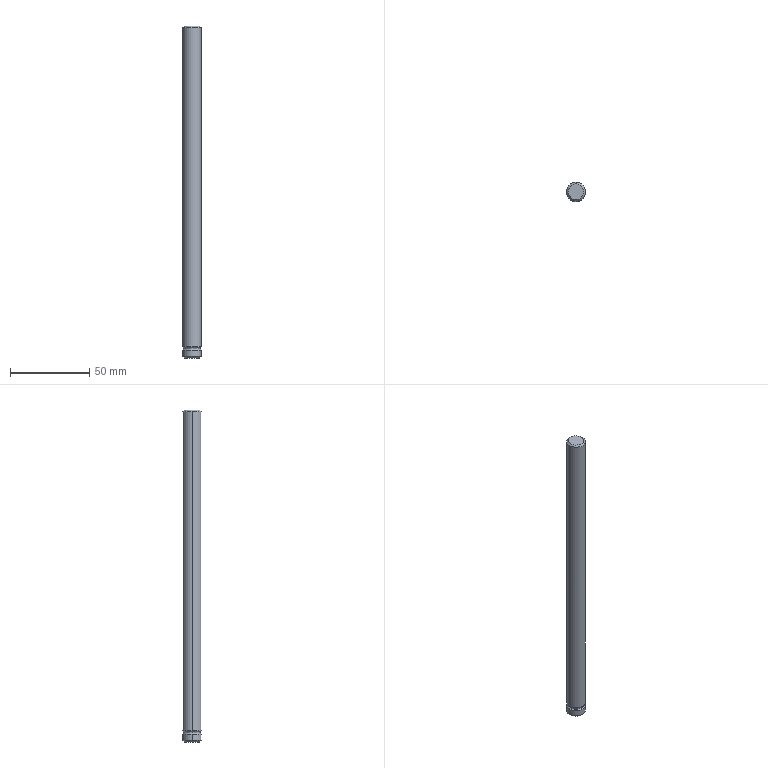Part | STEP file | Rotor mis-part check fixture-guide rod | 1 solid | 16 faces | box 12 x 12 x 210 mm | volume 23681 mm3 | cone 8 | cylinder 4 | spline 2 | plane 2 | commonest cylinder face diameters 12 x4
STEP:
#1=CARTESIAN_POINT('',(0.,0.,0.));
#2=DIRECTION('',(0.,0.,1.));
#3=DIRECTION('',(1.,0.,0.));
#4=AXIS2_PLACEMENT_3D('',#1,#2,#3);
#5=CARTESIAN_POINT('',(-5.354,0.,6.354));
#6=VERTEX_POINT('',#5);
#7=CARTESIAN_POINT('',(-5.354,0.,5.646));
#8=VERTEX_POINT('',#7);
#9=CARTESIAN_POINT('',(-5.707,0.,6.));
#10=DIRECTION('',(0.,1.,0.));
#11=DIRECTION('',(-1.,0.,0.));
#12=AXIS2_PLACEMENT_3D('',#9,#10,#11);
#13=CIRCLE('',#12,0.5);
#14=CARTESIAN_POINT('',(-5.354,0.,6.354));
#15=CARTESIAN_POINT('',(-5.354,10.707,6.354));
#16=CARTESIAN_POINT('',(5.354,10.707,6.354));
#17=CARTESIAN_POINT('',(5.354,0.,6.354));
#18=CARTESIAN_POINT('',(-5.146,0.,6.146));
#19=CARTESIAN_POINT('',(-5.146,10.293,6.146));
#20=CARTESIAN_POINT('',(5.146,10.293,6.146));
#21=CARTESIAN_POINT('',(5.146,0.,6.146));
#22=CARTESIAN_POINT('',(-5.146,0.,5.854));
#23=CARTESIAN_POINT('',(-5.146,10.293,5.854));
#24=CARTESIAN_POINT('',(5.146,10.293,5.854));
#25=CARTESIAN_POINT('',(5.146,0.,5.854));
#26=CARTESIAN_POINT('',(-5.354,0.,5.646));
#27=CARTESIAN_POINT('',(-5.354,10.707,5.646));
#28=CARTESIAN_POINT('',(5.354,10.707,5.646));
#29=CARTESIAN_POINT('',(5.354,0.,5.646));
#30=(BOUNDED_SURFACE()B_SPLINE_SURFACE(3,3,((#14,#15,#16,#17),(#18,#19,#20,#21),(#22,#23,#24,#25),(#26,#27,#28,#29)),.UNSPECIFIED.,.F.,.F.,.F.)B_SPLINE_SURFACE_WITH_KNOTS((4,4),(4,4),(0.,1.),(0.,1.),.PIECEWISE_BEZIER_KNOTS.)GEOMETRIC_REPRESENTATION_ITEM()RATIONAL_B_SPLINE_SURFACE(((1.,0.3333,0.3333,1.),(0.8047,0.2682,0.2682,0.8047),(0.8047,0.2682,0.2682,0.8047),(1.,0.3333,0.3333,1.)))REPRESENTATION_ITEM('')SURFACE());
#31=CARTESIAN_POINT('',(0.,0.));
#32=CARTESIAN_POINT('',(0.01683,0.));
#33=CARTESIAN_POINT('',(0.04999,0.));
#34=CARTESIAN_POINT('',(0.09843,0.));
#35=CARTESIAN_POINT('',(0.1457,0.));
#36=CARTESIAN_POINT('',(0.192,0.));
#37=CARTESIAN_POINT('',(0.2375,0.));
#38=CARTESIAN_POINT('',(0.2823,0.));
#39=CARTESIAN_POINT('',(0.3265,0.));
#40=CARTESIAN_POINT('',(0.3703,0.));
#41=CARTESIAN_POINT('',(0.4137,0.));
#42=CARTESIAN_POINT('',(0.4569,0.));
#43=CARTESIAN_POINT('',(0.5,0.));
#44=CARTESIAN_POINT('',(0.5431,0.));
#45=CARTESIAN_POINT('',(0.5863,0.));
#46=CARTESIAN_POINT('',(0.6297,0.));
#47=CARTESIAN_POINT('',(0.6735,0.));
#48=CARTESIAN_POINT('',(0.7177,0.));
#49=CARTESIAN_POINT('',(0.7625,0.));
#50=CARTESIAN_POINT('',(0.808,0.));
#51=CARTESIAN_POINT('',(0.8543,0.));
#52=CARTESIAN_POINT('',(0.9016,0.));
#53=CARTESIAN_POINT('',(0.95,0.));
#54=CARTESIAN_POINT('',(0.9832,0.));
#55=CARTESIAN_POINT('',(1.,0.));
#56=B_SPLINE_CURVE_WITH_KNOTS('',3,(#31,#32,#33,#34,#35,#36,#37,#38,#39,#40,#41,#42,#43,#44,#45,#46,#47,#48,#49,#50,#51,#52,#53,#54,#55),.UNSPECIFIED.,.F.,.F.,(4,1,1,1,1,1,1,1,1,1,1,1,1,1,1,1,1,1,1,1,1,1,4),(2.356,2.428,2.499,2.57,2.642,2.713,2.785,2.856,2.927,2.999,3.07,3.142,3.213,3.284,3.356,3.427,3.499,3.57,3.641,3.713,3.784,3.856,3.927),.QUASI_UNIFORM_KNOTS.);
#57=(GEOMETRIC_REPRESENTATION_CONTEXT(2)PARAMETRIC_REPRESENTATION_CONTEXT()REPRESENTATION_CONTEXT('',''));
#58=DEFINITIONAL_REPRESENTATION('',(#56),#57);
#59=PCURVE('',#30,#58);
#60=CARTESIAN_POINT('',(5.354,0.,6.354));
#61=CARTESIAN_POINT('',(5.354,-10.707,6.354));
#62=CARTESIAN_POINT('',(-5.354,-10.707,6.354));
#63=CARTESIAN_POINT('',(-5.354,0.,6.354));
#64=CARTESIAN_POINT('',(5.146,0.,6.146));
#65=CARTESIAN_POINT('',(5.146,-10.293,6.146));
#66=CARTESIAN_POINT('',(-5.146,-10.293,6.146));
#67=CARTESIAN_POINT('',(-5.146,0.,6.146));
#68=CARTESIAN_POINT('',(5.146,0.,5.854));
#69=CARTESIAN_POINT('',(5.146,-10.293,5.854));
#70=CARTESIAN_POINT('',(-5.146,-10.293,5.854));
#71=CARTESIAN_POINT('',(-5.146,0.,5.854));
#72=CARTESIAN_POINT('',(5.354,0.,5.646));
#73=CARTESIAN_POINT('',(5.354,-10.707,5.646));
#74=CARTESIAN_POINT('',(-5.354,-10.707,5.646));
#75=CARTESIAN_POINT('',(-5.354,0.,5.646));
#76=(BOUNDED_SURFACE()B_SPLINE_SURFACE(3,3,((#60,#61,#62,#63),(#64,#65,#66,#67),(#68,#69,#70,#71),(#72,#73,#74,#75)),.UNSPECIFIED.,.F.,.F.,.F.)B_SPLINE_SURFACE_WITH_KNOTS((4,4),(4,4),(0.,1.),(0.,1.),.PIECEWISE_BEZIER_KNOTS.)GEOMETRIC_REPRESENTATION_ITEM()RATIONAL_B_SPLINE_SURFACE(((1.,0.3333,0.3333,1.),(0.8047,0.2682,0.2682,0.8047),(0.8047,0.2682,0.2682,0.8047),(1.,0.3333,0.3333,1.)))REPRESENTATION_ITEM('')SURFACE());
#77=CARTESIAN_POINT('',(0.,1.));
#78=CARTESIAN_POINT('',(0.01683,1.));
#79=CARTESIAN_POINT('',(0.04999,1.));
#80=CARTESIAN_POINT('',(0.09843,1.));
#81=CARTESIAN_POINT('',(0.1457,1.));
#82=CARTESIAN_POINT('',(0.192,1.));
#83=CARTESIAN_POINT('',(0.2375,1.));
#84=CARTESIAN_POINT('',(0.2823,1.));
#85=CARTESIAN_POINT('',(0.3265,1.));
#86=CARTESIAN_POINT('',(0.3703,1.));
#87=CARTESIAN_POINT('',(0.4137,1.));
#88=CARTESIAN_POINT('',(0.4569,1.));
#89=CARTESIAN_POINT('',(0.5,1.));
#90=CARTESIAN_POINT('',(0.5431,1.));
#91=CARTESIAN_POINT('',(0.5863,1.));
#92=CARTESIAN_POINT('',(0.6297,1.));
#93=CARTESIAN_POINT('',(0.6735,1.));
#94=CARTESIAN_POINT('',(0.7177,1.));
#95=CARTESIAN_POINT('',(0.7625,1.));
#96=CARTESIAN_POINT('',(0.808,1.));
#97=CARTESIAN_POINT('',(0.8543,1.));
#98=CARTESIAN_POINT('',(0.9016,1.));
#99=CARTESIAN_POINT('',(0.95,1.));
#100=CARTESIAN_POINT('',(0.9832,1.));
#101=CARTESIAN_POINT('',(1.,1.));
#102=B_SPLINE_CURVE_WITH_KNOTS('',3,(#77,#78,#79,#80,#81,#82,#83,#84,#85,#86,#87,#88,#89,#90,#91,#92,#93,#94,#95,#96,#97,#98,#99,#100,#101),.UNSPECIFIED.,.F.,.F.,(4,1,1,1,1,1,1,1,1,1,1,1,1,1,1,1,1,1,1,1,1,1,4),(2.356,2.428,2.499,2.57,2.642,2.713,2.785,2.856,2.927,2.999,3.07,3.142,3.213,3.284,3.356,3.427,3.499,3.57,3.641,3.713,3.784,3.856,3.927),.QUASI_UNIFORM_KNOTS.);
#103=(GEOMETRIC_REPRESENTATION_CONTEXT(2)PARAMETRIC_REPRESENTATION_CONTEXT()REPRESENTATION_CONTEXT('',''));
#104=DEFINITIONAL_REPRESENTATION('',(#102),#103);
#105=PCURVE('',#76,#104);
#106=SURFACE_CURVE('',#13,(#59,#105),.PCURVE_S1.);
#107=EDGE_CURVE('',#6,#8,#106,.T.);
#108=ORIENTED_EDGE('',*,*,#107,.T.);
#109=CARTESIAN_POINT('',(5.354,0.,5.646));
#110=VERTEX_POINT('',#109);
#111=CARTESIAN_POINT('',(0.,0.,5.646));
#112=DIRECTION('',(0.,0.,-1.));
#113=DIRECTION('',(-1.,0.,0.));
#114=AXIS2_PLACEMENT_3D('',#111,#112,#113);
#115=CIRCLE('',#114,5.354);
#116=CARTESIAN_POINT('',(1.,0.));
#117=CARTESIAN_POINT('',(1.,0.02375));
#118=CARTESIAN_POINT('',(1.,0.06805));
#119=CARTESIAN_POINT('',(1.,0.1267));
#120=CARTESIAN_POINT('',(1.,0.1794));
#121=CARTESIAN_POINT('',(1.,0.2276));
#122=CARTESIAN_POINT('',(1.,0.2721));
#123=CARTESIAN_POINT('',(1.,0.3139));
#124=CARTESIAN_POINT('',(1.,0.3535));
#125=CARTESIAN_POINT('',(1.,0.3914));
#126=CARTESIAN_POINT('',(1.,0.4282));
#127=CARTESIAN_POINT('',(1.,0.4643));
#128=CARTESIAN_POINT('',(1.,0.5));
#129=CARTESIAN_POINT('',(1.,0.5357));
#130=CARTESIAN_POINT('',(1.,0.5718));
#131=CARTESIAN_POINT('',(1.,0.6086));
#132=CARTESIAN_POINT('',(1.,0.6465));
#133=CARTESIAN_POINT('',(1.,0.6861));
#134=CARTESIAN_POINT('',(1.,0.7279));
#135=CARTESIAN_POINT('',(1.,0.7724));
#136=CARTESIAN_POINT('',(1.,0.8206));
#137=CARTESIAN_POINT('',(1.,0.8733));
#138=CARTESIAN_POINT('',(1.,0.9319));
#139=CARTESIAN_POINT('',(1.,0.9763));
#140=CARTESIAN_POINT('',(1.,1.));
#141=B_SPLINE_CURVE_WITH_KNOTS('',3,(#116,#117,#118,#119,#120,#121,#122,#123,#124,#125,#126,#127,#128,#129,#130,#131,#132,#133,#134,#135,#136,#137,#138,#139,#140),.UNSPECIFIED.,.F.,.F.,(4,1,1,1,1,1,1,1,1,1,1,1,1,1,1,1,1,1,1,1,1,1,4),(0.,0.1428,0.2856,0.4284,0.5712,0.714,0.8568,0.9996,1.142,1.285,1.428,1.571,1.714,1.856,1.999,2.142,2.285,2.428,2.57,2.713,2.856,2.999,3.142),.QUASI_UNIFORM_KNOTS.);
#142=(GEOMETRIC_REPRESENTATION_CONTEXT(2)PARAMETRIC_REPRESENTATION_CONTEXT()REPRESENTATION_CONTEXT('',''));
#143=DEFINITIONAL_REPRESENTATION('',(#141),#142);
#144=PCURVE('',#30,#143);
#145=CARTESIAN_POINT('',(0.,0.,5.));
#146=DIRECTION('',(0.,0.,-1.));
#147=DIRECTION('',(-1.,0.,0.));
#148=AXIS2_PLACEMENT_3D('',#145,#146,#147);
#149=CONICAL_SURFACE('',#148,6.,0.7854);
#150=CARTESIAN_POINT('',(0.,-0.6464));
#151=DIRECTION('',(1.,0.));
#152=VECTOR('',#151,1.);
#153=LINE('',#150,#152);
#154=(GEOMETRIC_REPRESENTATION_CONTEXT(2)PARAMETRIC_REPRESENTATION_CONTEXT()REPRESENTATION_CONTEXT('',''));
#155=DEFINITIONAL_REPRESENTATION('',(#153),#154);
#156=PCURVE('',#149,#155);
#157=SURFACE_CURVE('',#115,(#144,#156),.PCURVE_S1.);
#158=EDGE_CURVE('',#8,#110,#157,.T.);
#159=ORIENTED_EDGE('',*,*,#158,.T.);
#160=CARTESIAN_POINT('',(5.354,0.,6.354));
#161=VERTEX_POINT('',#160);
#162=CARTESIAN_POINT('',(5.707,0.,6.));
#163=DIRECTION('',(0.,-1.,0.));
#164=DIRECTION('',(1.,0.,0.));
#165=AXIS2_PLACEMENT_3D('',#162,#163,#164);
#166=CIRCLE('',#165,0.5);
#167=CARTESIAN_POINT('',(0.,1.));
#168=CARTESIAN_POINT('',(0.01683,1.));
#169=CARTESIAN_POINT('',(0.04999,1.));
#170=CARTESIAN_POINT('',(0.09843,1.));
#171=CARTESIAN_POINT('',(0.1457,1.));
#172=CARTESIAN_POINT('',(0.192,1.));
#173=CARTESIAN_POINT('',(0.2375,1.));
#174=CARTESIAN_POINT('',(0.2823,1.));
#175=CARTESIAN_POINT('',(0.3265,1.));
#176=CARTESIAN_POINT('',(0.3703,1.));
#177=CARTESIAN_POINT('',(0.4137,1.));
#178=CARTESIAN_POINT('',(0.4569,1.));
#179=CARTESIAN_POINT('',(0.5,1.));
#180=CARTESIAN_POINT('',(0.5431,1.));
#181=CARTESIAN_POINT('',(0.5863,1.));
#182=CARTESIAN_POINT('',(0.6297,1.));
#183=CARTESIAN_POINT('',(0.6735,1.));
#184=CARTESIAN_POINT('',(0.7177,1.));
#185=CARTESIAN_POINT('',(0.7625,1.));
#186=CARTESIAN_POINT('',(0.808,1.));
#187=CARTESIAN_POINT('',(0.8543,1.));
#188=CARTESIAN_POINT('',(0.9016,1.));
#189=CARTESIAN_POINT('',(0.95,1.));
#190=CARTESIAN_POINT('',(0.9832,1.));
#191=CARTESIAN_POINT('',(1.,1.));
#192=B_SPLINE_CURVE_WITH_KNOTS('',3,(#167,#168,#169,#170,#171,#172,#173,#174,#175,#176,#177,#178,#179,#180,#181,#182,#183,#184,#185,#186,#187,#188,#189,#190,#191),.UNSPECIFIED.,.F.,.F.,(4,1,1,1,1,1,1,1,1,1,1,1,1,1,1,1,1,1,1,1,1,1,4),(2.356,2.428,2.499,2.57,2.642,2.713,2.785,2.856,2.927,2.999,3.07,3.142,3.213,3.284,3.356,3.427,3.499,3.57,3.641,3.713,3.784,3.856,3.927),.QUASI_UNIFORM_KNOTS.);
#193=(GEOMETRIC_REPRESENTATION_CONTEXT(2)PARAMETRIC_REPRESENTATION_CONTEXT()REPRESENTATION_CONTEXT('',''));
#194=DEFINITIONAL_REPRESENTATION('',(#192),#193);
#195=PCURVE('',#30,#194);
#196=CARTESIAN_POINT('',(0.,0.));
#197=CARTESIAN_POINT('',(0.01683,0.));
#198=CARTESIAN_POINT('',(0.04999,0.));
#199=CARTESIAN_POINT('',(0.09843,0.));
#200=CARTESIAN_POINT('',(0.1457,0.));
#201=CARTESIAN_POINT('',(0.192,0.));
#202=CARTESIAN_POINT('',(0.2375,0.));
#203=CARTESIAN_POINT('',(0.2823,0.));
#204=CARTESIAN_POINT('',(0.3265,0.));
#205=CARTESIAN_POINT('',(0.3703,0.));
#206=CARTESIAN_POINT('',(0.4137,0.));
#207=CARTESIAN_POINT('',(0.4569,0.));
#208=CARTESIAN_POINT('',(0.5,0.));
#209=CARTESIAN_POINT('',(0.5431,0.));
#210=CARTESIAN_POINT('',(0.5863,0.));
#211=CARTESIAN_POINT('',(0.6297,0.));
#212=CARTESIAN_POINT('',(0.6735,0.));
#213=CARTESIAN_POINT('',(0.7177,0.));
#214=CARTESIAN_POINT('',(0.7625,0.));
#215=CARTESIAN_POINT('',(0.808,0.));
#216=CARTESIAN_POINT('',(0.8543,0.));
#217=CARTESIAN_POINT('',(0.9016,0.));
#218=CARTESIAN_POINT('',(0.95,0.));
#219=CARTESIAN_POINT('',(0.9832,0.));
#220=CARTESIAN_POINT('',(1.,0.));
#221=B_SPLINE_CURVE_WITH_KNOTS('',3,(#196,#197,#198,#199,#200,#201,#202,#203,#204,#205,#206,#207,#208,#209,#210,#211,#212,#213,#214,#215,#216,#217,#218,#219,#220),.UNSPECIFIED.,.F.,.F.,(4,1,1,1,1,1,1,1,1,1,1,1,1,1,1,1,1,1,1,1,1,1,4),(2.356,2.428,2.499,2.57,2.642,2.713,2.785,2.856,2.927,2.999,3.07,3.142,3.213,3.284,3.356,3.427,3.499,3.57,3.641,3.713,3.784,3.856,3.927),.QUASI_UNIFORM_KNOTS.);
#222=(GEOMETRIC_REPRESENTATION_CONTEXT(2)PARAMETRIC_REPRESENTATION_CONTEXT()REPRESENTATION_CONTEXT('',''));
#223=DEFINITIONAL_REPRESENTATION('',(#221),#222);
#224=PCURVE('',#76,#223);
#225=SURFACE_CURVE('',#166,(#195,#224),.PCURVE_S1.);
#226=EDGE_CURVE('',#161,#110,#225,.T.);
#227=ORIENTED_EDGE('',*,*,#226,.F.);
#228=CARTESIAN_POINT('',(0.,0.,6.354));
#229=DIRECTION('',(0.,0.,1.));
#230=DIRECTION('',(1.,0.,0.));
#231=AXIS2_PLACEMENT_3D('',#228,#229,#230);
#232=CIRCLE('',#231,5.354);
#233=CARTESIAN_POINT('',(0.,1.));
#234=CARTESIAN_POINT('',(0.,0.9763));
#235=CARTESIAN_POINT('',(0.,0.9319));
#236=CARTESIAN_POINT('',(0.,0.8733));
#237=CARTESIAN_POINT('',(0.,0.8206));
#238=CARTESIAN_POINT('',(0.,0.7724));
#239=CARTESIAN_POINT('',(0.,0.7279));
#240=CARTESIAN_POINT('',(0.,0.6861));
#241=CARTESIAN_POINT('',(0.,0.6465));
#242=CARTESIAN_POINT('',(0.,0.6086));
#243=CARTESIAN_POINT('',(0.,0.5718));
#244=CARTESIAN_POINT('',(0.,0.5357));
#245=CARTESIAN_POINT('',(0.,0.5));
#246=CARTESIAN_POINT('',(0.,0.4643));
#247=CARTESIAN_POINT('',(0.,0.4282));
#248=CARTESIAN_POINT('',(0.,0.3914));
#249=CARTESIAN_POINT('',(0.,0.3535));
#250=CARTESIAN_POINT('',(0.,0.3139));
#251=CARTESIAN_POINT('',(0.,0.2721));
#252=CARTESIAN_POINT('',(0.,0.2276));
#253=CARTESIAN_POINT('',(0.,0.1794));
#254=CARTESIAN_POINT('',(0.,0.1267));
#255=CARTESIAN_POINT('',(0.,0.06805));
#256=CARTESIAN_POINT('',(0.,0.02375));
#257=CARTESIAN_POINT('',(0.,0.));
#258=B_SPLINE_CURVE_WITH_KNOTS('',3,(#233,#234,#235,#236,#237,#238,#239,#240,#241,#242,#243,#244,#245,#246,#247,#248,#249,#250,#251,#252,#253,#254,#255,#256,#257),.UNSPECIFIED.,.F.,.F.,(4,1,1,1,1,1,1,1,1,1,1,1,1,1,1,1,1,1,1,1,1,1,4),(0.,0.1428,0.2856,0.4284,0.5712,0.714,0.8568,0.9996,1.142,1.285,1.428,1.571,1.714,1.856,1.999,2.142,2.285,2.428,2.57,2.713,2.856,2.999,3.142),.QUASI_UNIFORM_KNOTS.);
#259=(GEOMETRIC_REPRESENTATION_CONTEXT(2)PARAMETRIC_REPRESENTATION_CONTEXT()REPRESENTATION_CONTEXT('',''));
#260=DEFINITIONAL_REPRESENTATION('',(#258),#259);
#261=PCURVE('',#30,#260);
#262=CARTESIAN_POINT('',(0.,0.,7.));
#263=DIRECTION('',(0.,0.,1.));
#264=DIRECTION('',(1.,0.,0.));
#265=AXIS2_PLACEMENT_3D('',#262,#263,#264);
#266=CONICAL_SURFACE('',#265,6.,0.7854);
#267=CARTESIAN_POINT('',(0.,-0.6464));
#268=DIRECTION('',(1.,0.));
#269=VECTOR('',#268,1.);
#270=LINE('',#267,#269);
#271=(GEOMETRIC_REPRESENTATION_CONTEXT(2)PARAMETRIC_REPRESENTATION_CONTEXT()REPRESENTATION_CONTEXT('',''));
#272=DEFINITIONAL_REPRESENTATION('',(#270),#271);
#273=PCURVE('',#266,#272);
#274=SURFACE_CURVE('',#232,(#261,#273),.PCURVE_S1.);
#275=EDGE_CURVE('',#161,#6,#274,.T.);
#276=ORIENTED_EDGE('',*,*,#275,.T.);
#277=EDGE_LOOP('',(#108,#159,#227,#276));
#278=FACE_BOUND('',#277,.F.);
#279=ADVANCED_FACE('',(#278),#30,.F.);
#280=CARTESIAN_POINT('',(-6.,0.,209.));
#281=VERTEX_POINT('',#280);
#282=CARTESIAN_POINT('',(6.,0.,209.));
#283=VERTEX_POINT('',#282);
#284=CARTESIAN_POINT('',(0.,0.,209.));
#285=DIRECTION('',(0.,0.,-1.));
#286=DIRECTION('',(-1.,0.,0.));
#287=AXIS2_PLACEMENT_3D('',#284,#285,#286);
#288=CIRCLE('',#287,6.);
#289=CARTESIAN_POINT('',(0.,0.,210.));
#290=DIRECTION('',(0.,0.,-1.));
#291=DIRECTION('',(-1.,0.,0.));
#292=AXIS2_PLACEMENT_3D('',#289,#290,#291);
#293=CYLINDRICAL_SURFACE('',#292,6.);
#294=CARTESIAN_POINT('',(0.,1.));
#295=DIRECTION('',(1.,0.));
#296=VECTOR('',#295,1.);
#297=LINE('',#294,#296);
#298=(GEOMETRIC_REPRESENTATION_CONTEXT(2)PARAMETRIC_REPRESENTATION_CONTEXT()REPRESENTATION_CONTEXT('',''));
#299=DEFINITIONAL_REPRESENTATION('',(#297),#298);
#300=PCURVE('',#293,#299);
#301=CARTESIAN_POINT('',(0.,0.,209.));
#302=DIRECTION('',(0.,0.,-1.));
#303=DIRECTION('',(-1.,0.,0.));
#304=AXIS2_PLACEMENT_3D('',#301,#302,#303);
#305=CONICAL_SURFACE('',#304,6.,0.7854);
#306=CARTESIAN_POINT('',(0.,0.));
#307=DIRECTION('',(1.,0.));
#308=VECTOR('',#307,1.);
#309=LINE('',#306,#308);
#310=(GEOMETRIC_REPRESENTATION_CONTEXT(2)PARAMETRIC_REPRESENTATION_CONTEXT()REPRESENTATION_CONTEXT('',''));
#311=DEFINITIONAL_REPRESENTATION('',(#309),#310);
#312=PCURVE('',#305,#311);
#313=SURFACE_CURVE('',#288,(#300,#312),.PCURVE_S1.);
#314=EDGE_CURVE('',#281,#283,#313,.T.);
#315=ORIENTED_EDGE('',*,*,#314,.T.);
#316=CARTESIAN_POINT('',(6.,0.,7.));
#317=VERTEX_POINT('',#316);
#318=CARTESIAN_POINT('',(6.,0.,210.));
#319=DIRECTION('',(0.,0.,-1.));
#320=VECTOR('',#319,1.);
#321=LINE('',#318,#320);
#322=CARTESIAN_POINT('',(3.142,0.));
#323=DIRECTION('',(0.,1.));
#324=VECTOR('',#323,1.);
#325=LINE('',#322,#324);
#326=(GEOMETRIC_REPRESENTATION_CONTEXT(2)PARAMETRIC_REPRESENTATION_CONTEXT()REPRESENTATION_CONTEXT('',''));
#327=DEFINITIONAL_REPRESENTATION('',(#325),#326);
#328=PCURVE('',#293,#327);
#329=CARTESIAN_POINT('',(0.,0.,210.));
#330=DIRECTION('',(0.,0.,-1.));
#331=DIRECTION('',(-1.,0.,0.));
#332=AXIS2_PLACEMENT_3D('',#329,#330,#331);
#333=CYLINDRICAL_SURFACE('',#332,6.);
#334=CARTESIAN_POINT('',(3.142,0.));
#335=DIRECTION('',(0.,1.));
#336=VECTOR('',#335,1.);
#337=LINE('',#334,#336);
#338=(GEOMETRIC_REPRESENTATION_CONTEXT(2)PARAMETRIC_REPRESENTATION_CONTEXT()REPRESENTATION_CONTEXT('',''));
#339=DEFINITIONAL_REPRESENTATION('',(#337),#338);
#340=PCURVE('',#333,#339);
#341=SURFACE_CURVE('',#321,(#328,#340),.PCURVE_S1.);
#342=EDGE_CURVE('',#283,#317,#341,.T.);
#343=ORIENTED_EDGE('',*,*,#342,.T.);
#344=CARTESIAN_POINT('',(-6.,0.,7.));
#345=VERTEX_POINT('',#344);
#346=CARTESIAN_POINT('',(0.,0.,7.));
#347=DIRECTION('',(0.,0.,1.));
#348=DIRECTION('',(-1.,0.,0.));
#349=AXIS2_PLACEMENT_3D('',#346,#347,#348);
#350=CIRCLE('',#349,6.);
#351=CARTESIAN_POINT('',(6.283,203.));
#352=DIRECTION('',(-1.,0.));
#353=VECTOR('',#352,1.);
#354=LINE('',#351,#353);
#355=(GEOMETRIC_REPRESENTATION_CONTEXT(2)PARAMETRIC_REPRESENTATION_CONTEXT()REPRESENTATION_CONTEXT('',''));
#356=DEFINITIONAL_REPRESENTATION('',(#354),#355);
#357=PCURVE('',#293,#356);
#358=CARTESIAN_POINT('',(-3.142,0.));
#359=DIRECTION('',(1.,0.));
#360=VECTOR('',#359,1.);
#361=LINE('',#358,#360);
#362=(GEOMETRIC_REPRESENTATION_CONTEXT(2)PARAMETRIC_REPRESENTATION_CONTEXT()REPRESENTATION_CONTEXT('',''));
#363=DEFINITIONAL_REPRESENTATION('',(#361),#362);
#364=PCURVE('',#266,#363);
#365=SURFACE_CURVE('',#350,(#357,#364),.PCURVE_S1.);
#366=EDGE_CURVE('',#317,#345,#365,.T.);
#367=ORIENTED_EDGE('',*,*,#366,.T.);
#368=CARTESIAN_POINT('',(-6.,0.,210.));
#369=DIRECTION('',(0.,0.,-1.));
#370=VECTOR('',#369,1.);
#371=LINE('',#368,#370);
#372=CARTESIAN_POINT('',(0.,0.));
#373=DIRECTION('',(0.,1.));
#374=VECTOR('',#373,1.);
#375=LINE('',#372,#374);
#376=(GEOMETRIC_REPRESENTATION_CONTEXT(2)PARAMETRIC_REPRESENTATION_CONTEXT()REPRESENTATION_CONTEXT('',''));
#377=DEFINITIONAL_REPRESENTATION('',(#375),#376);
#378=PCURVE('',#293,#377);
#379=CARTESIAN_POINT('',(6.283,0.));
#380=DIRECTION('',(0.,1.));
#381=VECTOR('',#380,1.);
#382=LINE('',#379,#381);
#383=(GEOMETRIC_REPRESENTATION_CONTEXT(2)PARAMETRIC_REPRESENTATION_CONTEXT()REPRESENTATION_CONTEXT('',''));
#384=DEFINITIONAL_REPRESENTATION('',(#382),#383);
#385=PCURVE('',#333,#384);
#386=SURFACE_CURVE('',#371,(#378,#385),.PCURVE_S1.);
#387=EDGE_CURVE('',#281,#345,#386,.T.);
#388=ORIENTED_EDGE('',*,*,#387,.F.);
#389=EDGE_LOOP('',(#315,#343,#367,#388));
#390=FACE_BOUND('',#389,.T.);
#391=ADVANCED_FACE('',(#390),#293,.T.);
#392=ORIENTED_EDGE('',*,*,#275,.T.);
#393=CARTESIAN_POINT('',(-6.,0.,7.));
#394=DIRECTION('',(-0.7071,0.,0.7071));
#395=VECTOR('',#394,1.);
#396=LINE('',#393,#395);
#397=CARTESIAN_POINT('',(3.142,0.));
#398=DIRECTION('',(0.,1.));
#399=VECTOR('',#398,1.);
#400=LINE('',#397,#399);
#401=(GEOMETRIC_REPRESENTATION_CONTEXT(2)PARAMETRIC_REPRESENTATION_CONTEXT()REPRESENTATION_CONTEXT('',''));
#402=DEFINITIONAL_REPRESENTATION('',(#400),#401);
#403=PCURVE('',#266,#402);
#404=CARTESIAN_POINT('',(0.,0.,7.));
#405=DIRECTION('',(0.,0.,1.));
#406=DIRECTION('',(1.,0.,0.));
#407=AXIS2_PLACEMENT_3D('',#404,#405,#406);
#408=CONICAL_SURFACE('',#407,6.,0.7854);
#409=CARTESIAN_POINT('',(3.142,0.));
#410=DIRECTION('',(0.,1.));
#411=VECTOR('',#410,1.);
#412=LINE('',#409,#411);
#413=(GEOMETRIC_REPRESENTATION_CONTEXT(2)PARAMETRIC_REPRESENTATION_CONTEXT()REPRESENTATION_CONTEXT('',''));
#414=DEFINITIONAL_REPRESENTATION('',(#412),#413);
#415=PCURVE('',#408,#414);
#416=SURFACE_CURVE('',#396,(#403,#415),.PCURVE_S1.);
#417=EDGE_CURVE('',#6,#345,#416,.T.);
#418=ORIENTED_EDGE('',*,*,#417,.T.);
#419=ORIENTED_EDGE('',*,*,#366,.F.);
#420=CARTESIAN_POINT('',(6.,0.,7.));
#421=DIRECTION('',(0.7071,0.,0.7071));
#422=VECTOR('',#421,1.);
#423=LINE('',#420,#422);
#424=CARTESIAN_POINT('',(0.,0.));
#425=DIRECTION('',(0.,1.));
#426=VECTOR('',#425,1.);
#427=LINE('',#424,#426);
#428=(GEOMETRIC_REPRESENTATION_CONTEXT(2)PARAMETRIC_REPRESENTATION_CONTEXT()REPRESENTATION_CONTEXT('',''));
#429=DEFINITIONAL_REPRESENTATION('',(#427),#428);
#430=PCURVE('',#266,#429);
#431=CARTESIAN_POINT('',(6.283,0.));
#432=DIRECTION('',(0.,1.));
#433=VECTOR('',#432,1.);
#434=LINE('',#431,#433);
#435=(GEOMETRIC_REPRESENTATION_CONTEXT(2)PARAMETRIC_REPRESENTATION_CONTEXT()REPRESENTATION_CONTEXT('',''));
#436=DEFINITIONAL_REPRESENTATION('',(#434),#435);
#437=PCURVE('',#408,#436);
#438=SURFACE_CURVE('',#423,(#430,#437),.PCURVE_S1.);
#439=EDGE_CURVE('',#161,#317,#438,.T.);
#440=ORIENTED_EDGE('',*,*,#439,.F.);
#441=EDGE_LOOP('',(#392,#418,#419,#440));
#442=FACE_BOUND('',#441,.T.);
#443=ADVANCED_FACE('',(#442),#266,.T.);
#444=CARTESIAN_POINT('',(-5.,0.,210.));
#445=VERTEX_POINT('',#444);
#446=CARTESIAN_POINT('',(5.,0.,210.));
#447=VERTEX_POINT('',#446);
#448=CARTESIAN_POINT('',(0.,0.,210.));
#449=DIRECTION('',(0.,0.,-1.));
#450=DIRECTION('',(-1.,0.,0.));
#451=AXIS2_PLACEMENT_3D('',#448,#449,#450);
#452=CIRCLE('',#451,5.);
#453=CARTESIAN_POINT('',(0.,-1.));
#454=DIRECTION('',(1.,0.));
#455=VECTOR('',#454,1.);
#456=LINE('',#453,#455);
#457=(GEOMETRIC_REPRESENTATION_CONTEXT(2)PARAMETRIC_REPRESENTATION_CONTEXT()REPRESENTATION_CONTEXT('',''));
#458=DEFINITIONAL_REPRESENTATION('',(#456),#457);
#459=PCURVE('',#305,#458);
#460=CARTESIAN_POINT('',(0.,0.,210.));
#461=DIRECTION('',(0.,0.,1.));
#462=DIRECTION('',(1.,0.,0.));
#463=AXIS2_PLACEMENT_3D('',#460,#461,#462);
#464=PLANE('',#463);
#465=CARTESIAN_POINT('',(-5.,0.));
#466=CARTESIAN_POINT('',(-5.,8.66));
#467=CARTESIAN_POINT('',(2.5,4.33));
#468=CARTESIAN_POINT('',(10.,0.));
#469=CARTESIAN_POINT('',(2.5,-4.33));
#470=CARTESIAN_POINT('',(-5.,-8.66));
#471=CARTESIAN_POINT('',(-5.,0.));
#472=(BOUNDED_CURVE()B_SPLINE_CURVE(2,(#465,#466,#467,#468,#469,#470,#471),.UNSPECIFIED.,.T.,.F.)B_SPLINE_CURVE_WITH_KNOTS((1,2,2,2,2,1),(-2.094,0.,2.094,4.189,6.283,8.378),.UNSPECIFIED.)CURVE()GEOMETRIC_REPRESENTATION_ITEM()RATIONAL_B_SPLINE_CURVE((1.,0.5,1.,0.5,1.,0.5,1.))REPRESENTATION_ITEM(''));
#473=(GEOMETRIC_REPRESENTATION_CONTEXT(2)PARAMETRIC_REPRESENTATION_CONTEXT()REPRESENTATION_CONTEXT('',''));
#474=DEFINITIONAL_REPRESENTATION('',(#472),#473);
#475=PCURVE('',#464,#474);
#476=SURFACE_CURVE('',#452,(#459,#475),.PCURVE_S1.);
#477=EDGE_CURVE('',#445,#447,#476,.T.);
#478=ORIENTED_EDGE('',*,*,#477,.T.);
#479=CARTESIAN_POINT('',(6.,0.,209.));
#480=DIRECTION('',(0.7071,0.,-0.7071));
#481=VECTOR('',#480,1.);
#482=LINE('',#479,#481);
#483=CARTESIAN_POINT('',(3.142,0.));
#484=DIRECTION('',(0.,1.));
#485=VECTOR('',#484,1.);
#486=LINE('',#483,#485);
#487=(GEOMETRIC_REPRESENTATION_CONTEXT(2)PARAMETRIC_REPRESENTATION_CONTEXT()REPRESENTATION_CONTEXT('',''));
#488=DEFINITIONAL_REPRESENTATION('',(#486),#487);
#489=PCURVE('',#305,#488);
#490=CARTESIAN_POINT('',(0.,0.,209.));
#491=DIRECTION('',(0.,0.,-1.));
#492=DIRECTION('',(-1.,0.,0.));
#493=AXIS2_PLACEMENT_3D('',#490,#491,#492);
#494=CONICAL_SURFACE('',#493,6.,0.7854);
#495=CARTESIAN_POINT('',(3.142,0.));
#496=DIRECTION('',(0.,1.));
#497=VECTOR('',#496,1.);
#498=LINE('',#495,#497);
#499=(GEOMETRIC_REPRESENTATION_CONTEXT(2)PARAMETRIC_REPRESENTATION_CONTEXT()REPRESENTATION_CONTEXT('',''));
#500=DEFINITIONAL_REPRESENTATION('',(#498),#499);
#501=PCURVE('',#494,#500);
#502=SURFACE_CURVE('',#482,(#489,#501),.PCURVE_S1.);
#503=EDGE_CURVE('',#447,#283,#502,.T.);
#504=ORIENTED_EDGE('',*,*,#503,.T.);
#505=ORIENTED_EDGE('',*,*,#314,.F.);
#506=CARTESIAN_POINT('',(-6.,0.,209.));
#507=DIRECTION('',(-0.7071,0.,-0.7071));
#508=VECTOR('',#507,1.);
#509=LINE('',#506,#508);
#510=CARTESIAN_POINT('',(0.,0.));
#511=DIRECTION('',(0.,1.));
#512=VECTOR('',#511,1.);
#513=LINE('',#510,#512);
#514=(GEOMETRIC_REPRESENTATION_CONTEXT(2)PARAMETRIC_REPRESENTATION_CONTEXT()REPRESENTATION_CONTEXT('',''));
#515=DEFINITIONAL_REPRESENTATION('',(#513),#514);
#516=PCURVE('',#305,#515);
#517=CARTESIAN_POINT('',(6.283,0.));
#518=DIRECTION('',(0.,1.));
#519=VECTOR('',#518,1.);
#520=LINE('',#517,#519);
#521=(GEOMETRIC_REPRESENTATION_CONTEXT(2)PARAMETRIC_REPRESENTATION_CONTEXT()REPRESENTATION_CONTEXT('',''));
#522=DEFINITIONAL_REPRESENTATION('',(#520),#521);
#523=PCURVE('',#494,#522);
#524=SURFACE_CURVE('',#509,(#516,#523),.PCURVE_S1.);
#525=EDGE_CURVE('',#445,#281,#524,.T.);
#526=ORIENTED_EDGE('',*,*,#525,.F.);
#527=EDGE_LOOP('',(#478,#504,#505,#526));
#528=FACE_BOUND('',#527,.T.);
#529=ADVANCED_FACE('',(#528),#305,.T.);
#530=ORIENTED_EDGE('',*,*,#158,.T.);
#531=CARTESIAN_POINT('',(6.,0.,5.));
#532=VERTEX_POINT('',#531);
#533=CARTESIAN_POINT('',(6.,0.,5.));
#534=DIRECTION('',(0.7071,0.,-0.7071));
#535=VECTOR('',#534,1.);
#536=LINE('',#533,#535);
#537=CARTESIAN_POINT('',(3.142,0.));
#538=DIRECTION('',(0.,1.));
#539=VECTOR('',#538,1.);
#540=LINE('',#537,#539);
#541=(GEOMETRIC_REPRESENTATION_CONTEXT(2)PARAMETRIC_REPRESENTATION_CONTEXT()REPRESENTATION_CONTEXT('',''));
#542=DEFINITIONAL_REPRESENTATION('',(#540),#541);
#543=PCURVE('',#149,#542);
#544=CARTESIAN_POINT('',(0.,0.,5.));
#545=DIRECTION('',(0.,0.,-1.));
#546=DIRECTION('',(-1.,0.,0.));
#547=AXIS2_PLACEMENT_3D('',#544,#545,#546);
#548=CONICAL_SURFACE('',#547,6.,0.7854);
#549=CARTESIAN_POINT('',(3.142,0.));
#550=DIRECTION('',(0.,1.));
#551=VECTOR('',#550,1.);
#552=LINE('',#549,#551);
#553=(GEOMETRIC_REPRESENTATION_CONTEXT(2)PARAMETRIC_REPRESENTATION_CONTEXT()REPRESENTATION_CONTEXT('',''));
#554=DEFINITIONAL_REPRESENTATION('',(#552),#553);
#555=PCURVE('',#548,#554);
#556=SURFACE_CURVE('',#536,(#543,#555),.PCURVE_S1.);
#557=EDGE_CURVE('',#110,#532,#556,.T.);
#558=ORIENTED_EDGE('',*,*,#557,.T.);
#559=CARTESIAN_POINT('',(-6.,0.,5.));
#560=VERTEX_POINT('',#559);
#561=CARTESIAN_POINT('',(0.,0.,5.));
#562=DIRECTION('',(0.,0.,1.));
#563=DIRECTION('',(-1.,0.,0.));
#564=AXIS2_PLACEMENT_3D('',#561,#562,#563);
#565=CIRCLE('',#564,6.);
#566=CARTESIAN_POINT('',(6.283,0.));
#567=DIRECTION('',(-1.,0.));
#568=VECTOR('',#567,1.);
#569=LINE('',#566,#568);
#570=(GEOMETRIC_REPRESENTATION_CONTEXT(2)PARAMETRIC_REPRESENTATION_CONTEXT()REPRESENTATION_CONTEXT('',''));
#571=DEFINITIONAL_REPRESENTATION('',(#569),#570);
#572=PCURVE('',#149,#571);
#573=CARTESIAN_POINT('',(0.,0.,210.));
#574=DIRECTION('',(0.,0.,-1.));
#575=DIRECTION('',(-1.,0.,0.));
#576=AXIS2_PLACEMENT_3D('',#573,#574,#575);
#577=CYLINDRICAL_SURFACE('',#576,6.);
#578=CARTESIAN_POINT('',(6.283,205.));
#579=DIRECTION('',(-1.,0.));
#580=VECTOR('',#579,1.);
#581=LINE('',#578,#580);
#582=(GEOMETRIC_REPRESENTATION_CONTEXT(2)PARAMETRIC_REPRESENTATION_CONTEXT()REPRESENTATION_CONTEXT('',''));
#583=DEFINITIONAL_REPRESENTATION('',(#581),#582);
#584=PCURVE('',#577,#583);
#585=SURFACE_CURVE('',#565,(#572,#584),.PCURVE_S1.);
#586=EDGE_CURVE('',#532,#560,#585,.T.);
#587=ORIENTED_EDGE('',*,*,#586,.T.);
#588=CARTESIAN_POINT('',(-6.,0.,5.));
#589=DIRECTION('',(-0.7071,0.,-0.7071));
#590=VECTOR('',#589,1.);
#591=LINE('',#588,#590);
#592=CARTESIAN_POINT('',(0.,0.));
#593=DIRECTION('',(0.,1.));
#594=VECTOR('',#593,1.);
#595=LINE('',#592,#594);
#596=(GEOMETRIC_REPRESENTATION_CONTEXT(2)PARAMETRIC_REPRESENTATION_CONTEXT()REPRESENTATION_CONTEXT('',''));
#597=DEFINITIONAL_REPRESENTATION('',(#595),#596);
#598=PCURVE('',#149,#597);
#599=CARTESIAN_POINT('',(6.283,0.));
#600=DIRECTION('',(0.,1.));
#601=VECTOR('',#600,1.);
#602=LINE('',#599,#601);
#603=(GEOMETRIC_REPRESENTATION_CONTEXT(2)PARAMETRIC_REPRESENTATION_CONTEXT()REPRESENTATION_CONTEXT('',''));
#604=DEFINITIONAL_REPRESENTATION('',(#602),#603);
#605=PCURVE('',#548,#604);
#606=SURFACE_CURVE('',#591,(#598,#605),.PCURVE_S1.);
#607=EDGE_CURVE('',#8,#560,#606,.T.);
#608=ORIENTED_EDGE('',*,*,#607,.F.);
#609=EDGE_LOOP('',(#530,#558,#587,#608));
#610=FACE_BOUND('',#609,.T.);
#611=ADVANCED_FACE('',(#610),#149,.T.);
#612=ORIENTED_EDGE('',*,*,#586,.F.);
#613=CARTESIAN_POINT('',(6.,0.,1.));
#614=VERTEX_POINT('',#613);
#615=CARTESIAN_POINT('',(6.,0.,210.));
#616=DIRECTION('',(0.,0.,-1.));
#617=VECTOR('',#616,1.);
#618=LINE('',#615,#617);
#619=CARTESIAN_POINT('',(3.142,0.));
#620=DIRECTION('',(0.,1.));
#621=VECTOR('',#620,1.);
#622=LINE('',#619,#621);
#623=(GEOMETRIC_REPRESENTATION_CONTEXT(2)PARAMETRIC_REPRESENTATION_CONTEXT()REPRESENTATION_CONTEXT('',''));
#624=DEFINITIONAL_REPRESENTATION('',(#622),#623);
#625=PCURVE('',#577,#624);
#626=CARTESIAN_POINT('',(0.,0.,210.));
#627=DIRECTION('',(0.,0.,-1.));
#628=DIRECTION('',(-1.,0.,0.));
#629=AXIS2_PLACEMENT_3D('',#626,#627,#628);
#630=CYLINDRICAL_SURFACE('',#629,6.);
#631=CARTESIAN_POINT('',(3.142,0.));
#632=DIRECTION('',(0.,1.));
#633=VECTOR('',#632,1.);
#634=LINE('',#631,#633);
#635=(GEOMETRIC_REPRESENTATION_CONTEXT(2)PARAMETRIC_REPRESENTATION_CONTEXT()REPRESENTATION_CONTEXT('',''));
#636=DEFINITIONAL_REPRESENTATION('',(#634),#635);
#637=PCURVE('',#630,#636);
#638=SURFACE_CURVE('',#618,(#625,#637),.PCURVE_S1.);
#639=EDGE_CURVE('',#532,#614,#638,.T.);
#640=ORIENTED_EDGE('',*,*,#639,.T.);
#641=CARTESIAN_POINT('',(-6.,0.,1.));
#642=VERTEX_POINT('',#641);
#643=CARTESIAN_POINT('',(0.,0.,1.));
#644=DIRECTION('',(0.,0.,1.));
#645=DIRECTION('',(-1.,0.,0.));
#646=AXIS2_PLACEMENT_3D('',#643,#644,#645);
#647=CIRCLE('',#646,6.);
#648=CARTESIAN_POINT('',(6.283,209.));
#649=DIRECTION('',(-1.,0.));
#650=VECTOR('',#649,1.);
#651=LINE('',#648,#650);
#652=(GEOMETRIC_REPRESENTATION_CONTEXT(2)PARAMETRIC_REPRESENTATION_CONTEXT()REPRESENTATION_CONTEXT('',''));
#653=DEFINITIONAL_REPRESENTATION('',(#651),#652);
#654=PCURVE('',#577,#653);
#655=CARTESIAN_POINT('',(0.,0.,1.));
#656=DIRECTION('',(0.,0.,1.));
#657=DIRECTION('',(1.,0.,0.));
#658=AXIS2_PLACEMENT_3D('',#655,#656,#657);
#659=CONICAL_SURFACE('',#658,6.,0.7854);
#660=CARTESIAN_POINT('',(-3.142,0.));
#661=DIRECTION('',(1.,0.));
#662=VECTOR('',#661,1.);
#663=LINE('',#660,#662);
#664=(GEOMETRIC_REPRESENTATION_CONTEXT(2)PARAMETRIC_REPRESENTATION_CONTEXT()REPRESENTATION_CONTEXT('',''));
#665=DEFINITIONAL_REPRESENTATION('',(#663),#664);
#666=PCURVE('',#659,#665);
#667=SURFACE_CURVE('',#647,(#654,#666),.PCURVE_S1.);
#668=EDGE_CURVE('',#614,#642,#667,.T.);
#669=ORIENTED_EDGE('',*,*,#668,.T.);
#670=CARTESIAN_POINT('',(-6.,0.,210.));
#671=DIRECTION('',(0.,0.,-1.));
#672=VECTOR('',#671,1.);
#673=LINE('',#670,#672);
#674=CARTESIAN_POINT('',(0.,0.));
#675=DIRECTION('',(0.,1.));
#676=VECTOR('',#675,1.);
#677=LINE('',#674,#676);
#678=(GEOMETRIC_REPRESENTATION_CONTEXT(2)PARAMETRIC_REPRESENTATION_CONTEXT()REPRESENTATION_CONTEXT('',''));
#679=DEFINITIONAL_REPRESENTATION('',(#677),#678);
#680=PCURVE('',#577,#679);
#681=CARTESIAN_POINT('',(6.283,0.));
#682=DIRECTION('',(0.,1.));
#683=VECTOR('',#682,1.);
#684=LINE('',#681,#683);
#685=(GEOMETRIC_REPRESENTATION_CONTEXT(2)PARAMETRIC_REPRESENTATION_CONTEXT()REPRESENTATION_CONTEXT('',''));
#686=DEFINITIONAL_REPRESENTATION('',(#684),#685);
#687=PCURVE('',#630,#686);
#688=SURFACE_CURVE('',#673,(#680,#687),.PCURVE_S1.);
#689=EDGE_CURVE('',#560,#642,#688,.T.);
#690=ORIENTED_EDGE('',*,*,#689,.F.);
#691=EDGE_LOOP('',(#612,#640,#669,#690));
#692=FACE_BOUND('',#691,.T.);
#693=ADVANCED_FACE('',(#692),#577,.T.);
#694=CARTESIAN_POINT('',(5.,0.,0.));
#695=VERTEX_POINT('',#694);
#696=CARTESIAN_POINT('',(-5.,0.,0.));
#697=VERTEX_POINT('',#696);
#698=CARTESIAN_POINT('',(0.,0.,0.));
#699=DIRECTION('',(0.,0.,1.));
#700=DIRECTION('',(1.,0.,0.));
#701=AXIS2_PLACEMENT_3D('',#698,#699,#700);
#702=CIRCLE('',#701,5.);
#703=CARTESIAN_POINT('',(0.,-1.));
#704=DIRECTION('',(1.,0.));
#705=VECTOR('',#704,1.);
#706=LINE('',#703,#705);
#707=(GEOMETRIC_REPRESENTATION_CONTEXT(2)PARAMETRIC_REPRESENTATION_CONTEXT()REPRESENTATION_CONTEXT('',''));
#708=DEFINITIONAL_REPRESENTATION('',(#706),#707);
#709=PCURVE('',#659,#708);
#710=CARTESIAN_POINT('',(0.,0.,0.));
#711=DIRECTION('',(0.,0.,1.));
#712=DIRECTION('',(1.,0.,0.));
#713=AXIS2_PLACEMENT_3D('',#710,#711,#712);
#714=PLANE('',#713);
#715=CARTESIAN_POINT('',(0.,0.));
#716=DIRECTION('',(1.,0.));
#717=AXIS2_PLACEMENT_2D('',#715,#716);
#718=CIRCLE('',#717,5.);
#719=(GEOMETRIC_REPRESENTATION_CONTEXT(2)PARAMETRIC_REPRESENTATION_CONTEXT()REPRESENTATION_CONTEXT('',''));
#720=DEFINITIONAL_REPRESENTATION('',(#718),#719);
#721=PCURVE('',#714,#720);
#722=SURFACE_CURVE('',#702,(#709,#721),.PCURVE_S1.);
#723=EDGE_CURVE('',#695,#697,#722,.T.);
#724=ORIENTED_EDGE('',*,*,#723,.T.);
#725=CARTESIAN_POINT('',(-6.,0.,1.));
#726=DIRECTION('',(-0.7071,0.,0.7071));
#727=VECTOR('',#726,1.);
#728=LINE('',#725,#727);
#729=CARTESIAN_POINT('',(3.142,0.));
#730=DIRECTION('',(0.,1.));
#731=VECTOR('',#730,1.);
#732=LINE('',#729,#731);
#733=(GEOMETRIC_REPRESENTATION_CONTEXT(2)PARAMETRIC_REPRESENTATION_CONTEXT()REPRESENTATION_CONTEXT('',''));
#734=DEFINITIONAL_REPRESENTATION('',(#732),#733);
#735=PCURVE('',#659,#734);
#736=CARTESIAN_POINT('',(0.,0.,1.));
#737=DIRECTION('',(0.,0.,1.));
#738=DIRECTION('',(1.,0.,0.));
#739=AXIS2_PLACEMENT_3D('',#736,#737,#738);
#740=CONICAL_SURFACE('',#739,6.,0.7854);
#741=CARTESIAN_POINT('',(3.142,0.));
#742=DIRECTION('',(0.,1.));
#743=VECTOR('',#742,1.);
#744=LINE('',#741,#743);
#745=(GEOMETRIC_REPRESENTATION_CONTEXT(2)PARAMETRIC_REPRESENTATION_CONTEXT()REPRESENTATION_CONTEXT('',''));
#746=DEFINITIONAL_REPRESENTATION('',(#744),#745);
#747=PCURVE('',#740,#746);
#748=SURFACE_CURVE('',#728,(#735,#747),.PCURVE_S1.);
#749=EDGE_CURVE('',#697,#642,#748,.T.);
#750=ORIENTED_EDGE('',*,*,#749,.T.);
#751=ORIENTED_EDGE('',*,*,#668,.F.);
#752=CARTESIAN_POINT('',(6.,0.,1.));
#753=DIRECTION('',(0.7071,0.,0.7071));
#754=VECTOR('',#753,1.);
#755=LINE('',#752,#754);
#756=CARTESIAN_POINT('',(0.,0.));
#757=DIRECTION('',(0.,1.));
#758=VECTOR('',#757,1.);
#759=LINE('',#756,#758);
#760=(GEOMETRIC_REPRESENTATION_CONTEXT(2)PARAMETRIC_REPRESENTATION_CONTEXT()REPRESENTATION_CONTEXT('',''));
#761=DEFINITIONAL_REPRESENTATION('',(#759),#760);
#762=PCURVE('',#659,#761);
#763=CARTESIAN_POINT('',(6.283,0.));
#764=DIRECTION('',(0.,1.));
#765=VECTOR('',#764,1.);
#766=LINE('',#763,#765);
#767=(GEOMETRIC_REPRESENTATION_CONTEXT(2)PARAMETRIC_REPRESENTATION_CONTEXT()REPRESENTATION_CONTEXT('',''));
#768=DEFINITIONAL_REPRESENTATION('',(#766),#767);
#769=PCURVE('',#740,#768);
#770=SURFACE_CURVE('',#755,(#762,#769),.PCURVE_S1.);
#771=EDGE_CURVE('',#695,#614,#770,.T.);
#772=ORIENTED_EDGE('',*,*,#771,.F.);
#773=EDGE_LOOP('',(#724,#750,#751,#772));
#774=FACE_BOUND('',#773,.T.);
#775=ADVANCED_FACE('',(#774),#659,.T.);
#776=ORIENTED_EDGE('',*,*,#342,.F.);
#777=CARTESIAN_POINT('',(0.,0.,209.));
#778=DIRECTION('',(0.,0.,-1.));
#779=DIRECTION('',(-1.,0.,0.));
#780=AXIS2_PLACEMENT_3D('',#777,#778,#779);
#781=CIRCLE('',#780,6.);
#782=CARTESIAN_POINT('',(0.,1.));
#783=DIRECTION('',(1.,0.));
#784=VECTOR('',#783,1.);
#785=LINE('',#782,#784);
#786=(GEOMETRIC_REPRESENTATION_CONTEXT(2)PARAMETRIC_REPRESENTATION_CONTEXT()REPRESENTATION_CONTEXT('',''));
#787=DEFINITIONAL_REPRESENTATION('',(#785),#786);
#788=PCURVE('',#333,#787);
#789=CARTESIAN_POINT('',(0.,0.));
#790=DIRECTION('',(1.,0.));
#791=VECTOR('',#790,1.);
#792=LINE('',#789,#791);
#793=(GEOMETRIC_REPRESENTATION_CONTEXT(2)PARAMETRIC_REPRESENTATION_CONTEXT()REPRESENTATION_CONTEXT('',''));
#794=DEFINITIONAL_REPRESENTATION('',(#792),#793);
#795=PCURVE('',#494,#794);
#796=SURFACE_CURVE('',#781,(#788,#795),.PCURVE_S1.);
#797=EDGE_CURVE('',#283,#281,#796,.T.);
#798=ORIENTED_EDGE('',*,*,#797,.T.);
#799=ORIENTED_EDGE('',*,*,#387,.T.);
#800=CARTESIAN_POINT('',(0.,0.,7.));
#801=DIRECTION('',(0.,0.,1.));
#802=DIRECTION('',(-1.,0.,0.));
#803=AXIS2_PLACEMENT_3D('',#800,#801,#802);
#804=CIRCLE('',#803,6.);
#805=CARTESIAN_POINT('',(6.283,203.));
#806=DIRECTION('',(-1.,0.));
#807=VECTOR('',#806,1.);
#808=LINE('',#805,#807);
#809=(GEOMETRIC_REPRESENTATION_CONTEXT(2)PARAMETRIC_REPRESENTATION_CONTEXT()REPRESENTATION_CONTEXT('',''));
#810=DEFINITIONAL_REPRESENTATION('',(#808),#809);
#811=PCURVE('',#333,#810);
#812=CARTESIAN_POINT('',(3.142,0.));
#813=DIRECTION('',(1.,0.));
#814=VECTOR('',#813,1.);
#815=LINE('',#812,#814);
#816=(GEOMETRIC_REPRESENTATION_CONTEXT(2)PARAMETRIC_REPRESENTATION_CONTEXT()REPRESENTATION_CONTEXT('',''));
#817=DEFINITIONAL_REPRESENTATION('',(#815),#816);
#818=PCURVE('',#408,#817);
#819=SURFACE_CURVE('',#804,(#811,#818),.PCURVE_S1.);
#820=EDGE_CURVE('',#345,#317,#819,.T.);
#821=ORIENTED_EDGE('',*,*,#820,.T.);
#822=EDGE_LOOP('',(#776,#798,#799,#821));
#823=FACE_BOUND('',#822,.T.);
#824=ADVANCED_FACE('',(#823),#333,.T.);
#825=ORIENTED_EDGE('',*,*,#417,.F.);
#826=CARTESIAN_POINT('',(0.,0.,6.354));
#827=DIRECTION('',(0.,0.,1.));
#828=DIRECTION('',(1.,0.,0.));
#829=AXIS2_PLACEMENT_3D('',#826,#827,#828);
#830=CIRCLE('',#829,5.354);
#831=CARTESIAN_POINT('',(0.,-0.6464));
#832=DIRECTION('',(1.,0.));
#833=VECTOR('',#832,1.);
#834=LINE('',#831,#833);
#835=(GEOMETRIC_REPRESENTATION_CONTEXT(2)PARAMETRIC_REPRESENTATION_CONTEXT()REPRESENTATION_CONTEXT('',''));
#836=DEFINITIONAL_REPRESENTATION('',(#834),#835);
#837=PCURVE('',#408,#836);
#838=CARTESIAN_POINT('',(0.,1.));
#839=CARTESIAN_POINT('',(0.,0.9763));
#840=CARTESIAN_POINT('',(0.,0.9319));
#841=CARTESIAN_POINT('',(0.,0.8733));
#842=CARTESIAN_POINT('',(0.,0.8206));
#843=CARTESIAN_POINT('',(0.,0.7724));
#844=CARTESIAN_POINT('',(0.,0.7279));
#845=CARTESIAN_POINT('',(0.,0.6861));
#846=CARTESIAN_POINT('',(0.,0.6465));
#847=CARTESIAN_POINT('',(0.,0.6086));
#848=CARTESIAN_POINT('',(0.,0.5718));
#849=CARTESIAN_POINT('',(0.,0.5357));
#850=CARTESIAN_POINT('',(0.,0.5));
#851=CARTESIAN_POINT('',(0.,0.4643));
#852=CARTESIAN_POINT('',(0.,0.4282));
#853=CARTESIAN_POINT('',(0.,0.3914));
#854=CARTESIAN_POINT('',(0.,0.3535));
#855=CARTESIAN_POINT('',(0.,0.3139));
#856=CARTESIAN_POINT('',(0.,0.2721));
#857=CARTESIAN_POINT('',(0.,0.2276));
#858=CARTESIAN_POINT('',(0.,0.1794));
#859=CARTESIAN_POINT('',(0.,0.1267));
#860=CARTESIAN_POINT('',(0.,0.06805));
#861=CARTESIAN_POINT('',(0.,0.02375));
#862=CARTESIAN_POINT('',(0.,0.));
#863=B_SPLINE_CURVE_WITH_KNOTS('',3,(#838,#839,#840,#841,#842,#843,#844,#845,#846,#847,#848,#849,#850,#851,#852,#853,#854,#855,#856,#857,#858,#859,#860,#861,#862),.UNSPECIFIED.,.F.,.F.,(4,1,1,1,1,1,1,1,1,1,1,1,1,1,1,1,1,1,1,1,1,1,4),(3.142,3.284,3.427,3.57,3.713,3.856,3.998,4.141,4.284,4.427,4.57,4.712,4.855,4.998,5.141,5.284,5.426,5.569,5.712,5.855,5.998,6.14,6.283),.QUASI_UNIFORM_KNOTS.);
#864=(GEOMETRIC_REPRESENTATION_CONTEXT(2)PARAMETRIC_REPRESENTATION_CONTEXT()REPRESENTATION_CONTEXT('',''));
#865=DEFINITIONAL_REPRESENTATION('',(#863),#864);
#866=PCURVE('',#76,#865);
#867=SURFACE_CURVE('',#830,(#837,#866),.PCURVE_S1.);
#868=EDGE_CURVE('',#6,#161,#867,.T.);
#869=ORIENTED_EDGE('',*,*,#868,.T.);
#870=ORIENTED_EDGE('',*,*,#439,.T.);
#871=ORIENTED_EDGE('',*,*,#820,.F.);
#872=EDGE_LOOP('',(#825,#869,#870,#871));
#873=FACE_BOUND('',#872,.T.);
#874=ADVANCED_FACE('',(#873),#408,.T.);
#875=ORIENTED_EDGE('',*,*,#503,.F.);
#876=CARTESIAN_POINT('',(0.,0.,210.));
#877=DIRECTION('',(0.,0.,-1.));
#878=DIRECTION('',(-1.,0.,0.));
#879=AXIS2_PLACEMENT_3D('',#876,#877,#878);
#880=CIRCLE('',#879,5.);
#881=CARTESIAN_POINT('',(0.,-1.));
#882=DIRECTION('',(1.,0.));
#883=VECTOR('',#882,1.);
#884=LINE('',#881,#883);
#885=(GEOMETRIC_REPRESENTATION_CONTEXT(2)PARAMETRIC_REPRESENTATION_CONTEXT()REPRESENTATION_CONTEXT('',''));
#886=DEFINITIONAL_REPRESENTATION('',(#884),#885);
#887=PCURVE('',#494,#886);
#888=CARTESIAN_POINT('',(-5.,0.));
#889=CARTESIAN_POINT('',(-5.,8.66));
#890=CARTESIAN_POINT('',(2.5,4.33));
#891=CARTESIAN_POINT('',(10.,0.));
#892=CARTESIAN_POINT('',(2.5,-4.33));
#893=CARTESIAN_POINT('',(-5.,-8.66));
#894=CARTESIAN_POINT('',(-5.,0.));
#895=(BOUNDED_CURVE()B_SPLINE_CURVE(2,(#888,#889,#890,#891,#892,#893,#894),.UNSPECIFIED.,.T.,.F.)B_SPLINE_CURVE_WITH_KNOTS((1,2,2,2,2,1),(-2.094,0.,2.094,4.189,6.283,8.378),.UNSPECIFIED.)CURVE()GEOMETRIC_REPRESENTATION_ITEM()RATIONAL_B_SPLINE_CURVE((1.,0.5,1.,0.5,1.,0.5,1.))REPRESENTATION_ITEM(''));
#896=(GEOMETRIC_REPRESENTATION_CONTEXT(2)PARAMETRIC_REPRESENTATION_CONTEXT()REPRESENTATION_CONTEXT('',''));
#897=DEFINITIONAL_REPRESENTATION('',(#895),#896);
#898=PCURVE('',#464,#897);
#899=SURFACE_CURVE('',#880,(#887,#898),.PCURVE_S1.);
#900=EDGE_CURVE('',#447,#445,#899,.T.);
#901=ORIENTED_EDGE('',*,*,#900,.T.);
#902=ORIENTED_EDGE('',*,*,#525,.T.);
#903=ORIENTED_EDGE('',*,*,#797,.F.);
#904=EDGE_LOOP('',(#875,#901,#902,#903));
#905=FACE_BOUND('',#904,.T.);
#906=ADVANCED_FACE('',(#905),#494,.T.);
#907=CARTESIAN_POINT('',(0.,0.,5.646));
#908=DIRECTION('',(0.,0.,-1.));
#909=DIRECTION('',(-1.,0.,0.));
#910=AXIS2_PLACEMENT_3D('',#907,#908,#909);
#911=CIRCLE('',#910,5.354);
#912=CARTESIAN_POINT('',(1.,0.));
#913=CARTESIAN_POINT('',(1.,0.02375));
#914=CARTESIAN_POINT('',(1.,0.06805));
#915=CARTESIAN_POINT('',(1.,0.1267));
#916=CARTESIAN_POINT('',(1.,0.1794));
#917=CARTESIAN_POINT('',(1.,0.2276));
#918=CARTESIAN_POINT('',(1.,0.2721));
#919=CARTESIAN_POINT('',(1.,0.3139));
#920=CARTESIAN_POINT('',(1.,0.3535));
#921=CARTESIAN_POINT('',(1.,0.3914));
#922=CARTESIAN_POINT('',(1.,0.4282));
#923=CARTESIAN_POINT('',(1.,0.4643));
#924=CARTESIAN_POINT('',(1.,0.5));
#925=CARTESIAN_POINT('',(1.,0.5357));
#926=CARTESIAN_POINT('',(1.,0.5718));
#927=CARTESIAN_POINT('',(1.,0.6086));
#928=CARTESIAN_POINT('',(1.,0.6465));
#929=CARTESIAN_POINT('',(1.,0.6861));
#930=CARTESIAN_POINT('',(1.,0.7279));
#931=CARTESIAN_POINT('',(1.,0.7724));
#932=CARTESIAN_POINT('',(1.,0.8206));
#933=CARTESIAN_POINT('',(1.,0.8733));
#934=CARTESIAN_POINT('',(1.,0.9319));
#935=CARTESIAN_POINT('',(1.,0.9763));
#936=CARTESIAN_POINT('',(1.,1.));
#937=B_SPLINE_CURVE_WITH_KNOTS('',3,(#912,#913,#914,#915,#916,#917,#918,#919,#920,#921,#922,#923,#924,#925,#926,#927,#928,#929,#930,#931,#932,#933,#934,#935,#936),.UNSPECIFIED.,.F.,.F.,(4,1,1,1,1,1,1,1,1,1,1,1,1,1,1,1,1,1,1,1,1,1,4),(3.142,3.284,3.427,3.57,3.713,3.856,3.998,4.141,4.284,4.427,4.57,4.712,4.855,4.998,5.141,5.284,5.426,5.569,5.712,5.855,5.998,6.14,6.283),.QUASI_UNIFORM_KNOTS.);
#938=(GEOMETRIC_REPRESENTATION_CONTEXT(2)PARAMETRIC_REPRESENTATION_CONTEXT()REPRESENTATION_CONTEXT('',''));
#939=DEFINITIONAL_REPRESENTATION('',(#937),#938);
#940=PCURVE('',#76,#939);
#941=CARTESIAN_POINT('',(0.,-0.6464));
#942=DIRECTION('',(1.,0.));
#943=VECTOR('',#942,1.);
#944=LINE('',#941,#943);
#945=(GEOMETRIC_REPRESENTATION_CONTEXT(2)PARAMETRIC_REPRESENTATION_CONTEXT()REPRESENTATION_CONTEXT('',''));
#946=DEFINITIONAL_REPRESENTATION('',(#944),#945);
#947=PCURVE('',#548,#946);
#948=SURFACE_CURVE('',#911,(#940,#947),.PCURVE_S1.);
#949=EDGE_CURVE('',#110,#8,#948,.T.);
#950=ORIENTED_EDGE('',*,*,#949,.T.);
#951=ORIENTED_EDGE('',*,*,#107,.F.);
#952=ORIENTED_EDGE('',*,*,#868,.T.);
#953=ORIENTED_EDGE('',*,*,#226,.T.);
#954=EDGE_LOOP('',(#950,#951,#952,#953));
#955=FACE_BOUND('',#954,.F.);
#956=ADVANCED_FACE('',(#955),#76,.F.);
#957=ORIENTED_EDGE('',*,*,#477,.F.);
#958=ORIENTED_EDGE('',*,*,#900,.F.);
#959=EDGE_LOOP('',(#957,#958));
#960=FACE_BOUND('',#959,.T.);
#961=ADVANCED_FACE('',(#960),#464,.T.);
#962=ORIENTED_EDGE('',*,*,#557,.F.);
#963=ORIENTED_EDGE('',*,*,#949,.T.);
#964=ORIENTED_EDGE('',*,*,#607,.T.);
#965=CARTESIAN_POINT('',(0.,0.,5.));
#966=DIRECTION('',(0.,0.,1.));
#967=DIRECTION('',(-1.,0.,0.));
#968=AXIS2_PLACEMENT_3D('',#965,#966,#967);
#969=CIRCLE('',#968,6.);
#970=CARTESIAN_POINT('',(6.283,0.));
#971=DIRECTION('',(-1.,0.));
#972=VECTOR('',#971,1.);
#973=LINE('',#970,#972);
#974=(GEOMETRIC_REPRESENTATION_CONTEXT(2)PARAMETRIC_REPRESENTATION_CONTEXT()REPRESENTATION_CONTEXT('',''));
#975=DEFINITIONAL_REPRESENTATION('',(#973),#974);
#976=PCURVE('',#548,#975);
#977=CARTESIAN_POINT('',(6.283,205.));
#978=DIRECTION('',(-1.,0.));
#979=VECTOR('',#978,1.);
#980=LINE('',#977,#979);
#981=(GEOMETRIC_REPRESENTATION_CONTEXT(2)PARAMETRIC_REPRESENTATION_CONTEXT()REPRESENTATION_CONTEXT('',''));
#982=DEFINITIONAL_REPRESENTATION('',(#980),#981);
#983=PCURVE('',#630,#982);
#984=SURFACE_CURVE('',#969,(#976,#983),.PCURVE_S1.);
#985=EDGE_CURVE('',#560,#532,#984,.T.);
#986=ORIENTED_EDGE('',*,*,#985,.T.);
#987=EDGE_LOOP('',(#962,#963,#964,#986));
#988=FACE_BOUND('',#987,.T.);
#989=ADVANCED_FACE('',(#988),#548,.T.);
#990=ORIENTED_EDGE('',*,*,#639,.F.);
#991=ORIENTED_EDGE('',*,*,#985,.F.);
#992=ORIENTED_EDGE('',*,*,#689,.T.);
#993=CARTESIAN_POINT('',(0.,0.,1.));
#994=DIRECTION('',(0.,0.,1.));
#995=DIRECTION('',(-1.,0.,0.));
#996=AXIS2_PLACEMENT_3D('',#993,#994,#995);
#997=CIRCLE('',#996,6.);
#998=CARTESIAN_POINT('',(6.283,209.));
#999=DIRECTION('',(-1.,0.));
#1000=VECTOR('',#999,1.);
#1001=LINE('',#998,#1000);
#1002=(GEOMETRIC_REPRESENTATION_CONTEXT(2)PARAMETRIC_REPRESENTATION_CONTEXT()REPRESENTATION_CONTEXT('',''));
#1003=DEFINITIONAL_REPRESENTATION('',(#1001),#1002);
#1004=PCURVE('',#630,#1003);
#1005=CARTESIAN_POINT('',(3.142,0.));
#1006=DIRECTION('',(1.,0.));
#1007=VECTOR('',#1006,1.);
#1008=LINE('',#1005,#1007);
#1009=(GEOMETRIC_REPRESENTATION_CONTEXT(2)PARAMETRIC_REPRESENTATION_CONTEXT()REPRESENTATION_CONTEXT('',''));
#1010=DEFINITIONAL_REPRESENTATION('',(#1008),#1009);
#1011=PCURVE('',#740,#1010);
#1012=SURFACE_CURVE('',#997,(#1004,#1011),.PCURVE_S1.);
#1013=EDGE_CURVE('',#642,#614,#1012,.T.);
#1014=ORIENTED_EDGE('',*,*,#1013,.T.);
#1015=EDGE_LOOP('',(#990,#991,#992,#1014));
#1016=FACE_BOUND('',#1015,.T.);
#1017=ADVANCED_FACE('',(#1016),#630,.T.);
#1018=ORIENTED_EDGE('',*,*,#749,.F.);
#1019=CARTESIAN_POINT('',(0.,0.,0.));
#1020=DIRECTION('',(0.,0.,1.));
#1021=DIRECTION('',(1.,0.,0.));
#1022=AXIS2_PLACEMENT_3D('',#1019,#1020,#1021);
#1023=CIRCLE('',#1022,5.);
#1024=CARTESIAN_POINT('',(0.,-1.));
#1025=DIRECTION('',(1.,0.));
#1026=VECTOR('',#1025,1.);
#1027=LINE('',#1024,#1026);
#1028=(GEOMETRIC_REPRESENTATION_CONTEXT(2)PARAMETRIC_REPRESENTATION_CONTEXT()REPRESENTATION_CONTEXT('',''));
#1029=DEFINITIONAL_REPRESENTATION('',(#1027),#1028);
#1030=PCURVE('',#740,#1029);
#1031=CARTESIAN_POINT('',(0.,0.));
#1032=DIRECTION('',(1.,0.));
#1033=AXIS2_PLACEMENT_2D('',#1031,#1032);
#1034=CIRCLE('',#1033,5.);
#1035=(GEOMETRIC_REPRESENTATION_CONTEXT(2)PARAMETRIC_REPRESENTATION_CONTEXT()REPRESENTATION_CONTEXT('',''));
#1036=DEFINITIONAL_REPRESENTATION('',(#1034),#1035);
#1037=PCURVE('',#714,#1036);
#1038=SURFACE_CURVE('',#1023,(#1030,#1037),.PCURVE_S1.);
#1039=EDGE_CURVE('',#697,#695,#1038,.T.);
#1040=ORIENTED_EDGE('',*,*,#1039,.T.);
#1041=ORIENTED_EDGE('',*,*,#771,.T.);
#1042=ORIENTED_EDGE('',*,*,#1013,.F.);
#1043=EDGE_LOOP('',(#1018,#1040,#1041,#1042));
#1044=FACE_BOUND('',#1043,.T.);
#1045=ADVANCED_FACE('',(#1044),#740,.T.);
#1046=ORIENTED_EDGE('',*,*,#723,.F.);
#1047=ORIENTED_EDGE('',*,*,#1039,.F.);
#1048=EDGE_LOOP('',(#1046,#1047));
#1049=FACE_BOUND('',#1048,.T.);
#1050=ADVANCED_FACE('',(#1049),#714,.F.);
#1051=CLOSED_SHELL('',(#279,#391,#443,#529,#611,#693,#775,#824,#874,#906,#956,#961,#989,#1017,#1045,#1050));
#1052=MANIFOLD_SOLID_BREP('',#1051);
#1053=(LENGTH_UNIT()NAMED_UNIT(*)SI_UNIT(.MILLI.,.METRE.));
#1054=UNCERTAINTY_MEASURE_WITH_UNIT(LENGTH_MEASURE(0.0000001),#1053,'','');
#1055=(NAMED_UNIT(*)PLANE_ANGLE_UNIT()SI_UNIT($,.RADIAN.));
#1056=(NAMED_UNIT(*)SI_UNIT($,.STERADIAN.)SOLID_ANGLE_UNIT());
#1057=(GEOMETRIC_REPRESENTATION_CONTEXT(3)GLOBAL_UNCERTAINTY_ASSIGNED_CONTEXT((#1054))GLOBAL_UNIT_ASSIGNED_CONTEXT((#1053,#1055,#1056))REPRESENTATION_CONTEXT('',''));
#1058=ADVANCED_BREP_SHAPE_REPRESENTATION('',(#4,#1052),#1057);